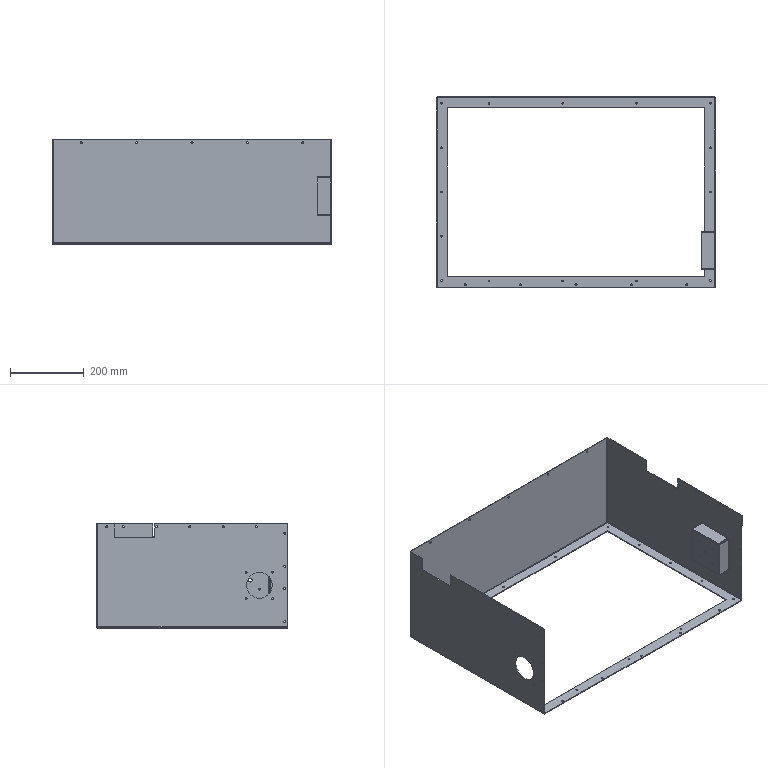Part | STEP file | MT-COMBO-119-S001_Default<Machined> | 1 solid | 200 faces | box 758 x 516.5 x 282.5 mm | volume 1425060 mm3 | cylinder 122 | plane 58 | spline 12 | cone 8 | commonest cylinder face diameters 5.5 x52 4.2 x34 4.5 x16 1.473 x8 6.473 x8 10 x2